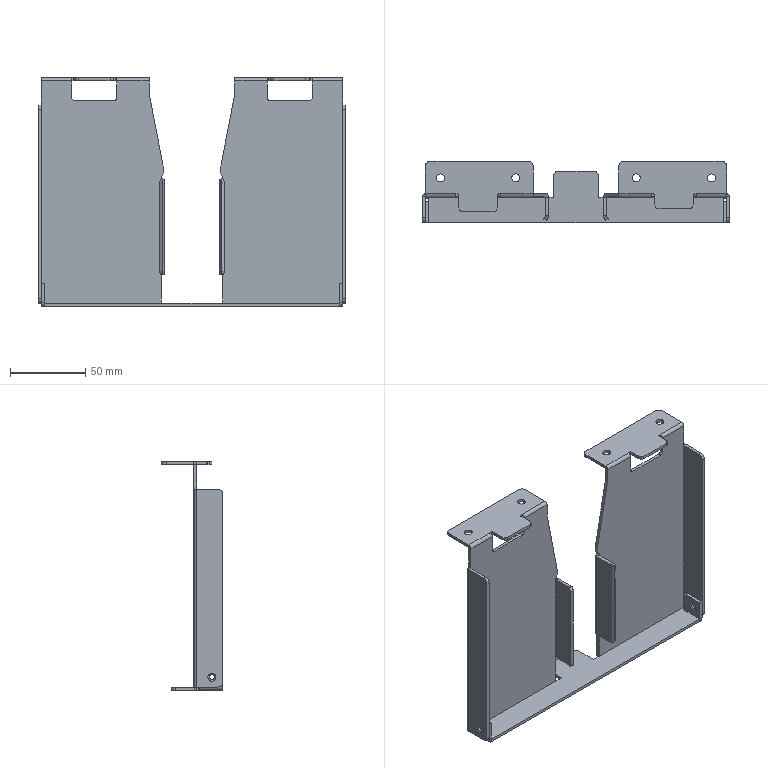Part | NX | features solid 2 | 1 solid | 204 faces | box 204 x 40.5 x 151.541 mm | volume 74907 mm3 | plane 118 | cylinder 74 | cone 8 | spline 4 | commonest cylinder face diameters 4 x24 2 x10 6 x10 3.3 x8 5.3 x8 0.4 x6